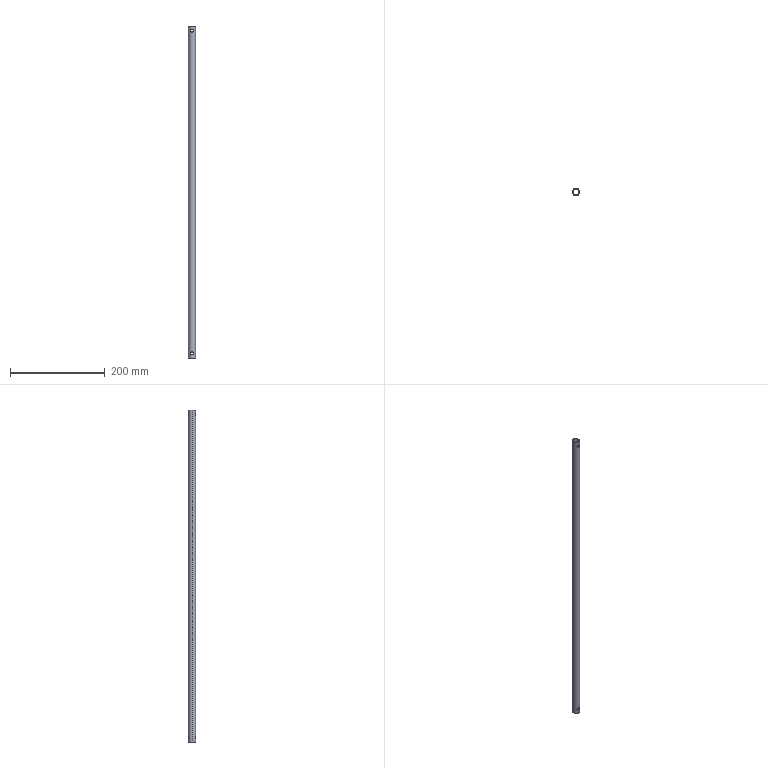Part | SolidWorks | features Extrusion 1, ICE 1 | 1 solid | 14 faces | box 15 x 15 x 700 mm | volume 44358 mm3 | cylinder 12 | plane 2 | commonest cylinder face diameters 6 x8 12 x2 15 x2
STEP:
#1=CARTESIAN_POINT('',(0.,-7.5,687.));
#2=VERTEX_POINT('',#1);
#3=CARTESIAN_POINT('',(0.,-7.5,693.));
#4=VERTEX_POINT('',#3);
#5=CARTESIAN_POINT('',(0.,-7.5,687.));
#6=CARTESIAN_POINT('',(-0.1973,-7.5,687.));
#7=CARTESIAN_POINT('',(-0.3974,-7.492,687.02));
#8=CARTESIAN_POINT('',(-0.7861,-7.461,687.098));
#9=CARTESIAN_POINT('',(-0.9739,-7.439,687.156));
#10=CARTESIAN_POINT('',(-1.337,-7.382,687.307));
#11=CARTESIAN_POINT('',(-1.511,-7.348,687.401));
#12=CARTESIAN_POINT('',(-1.834,-7.274,687.618));
#13=CARTESIAN_POINT('',(-1.985,-7.234,687.742));
#14=CARTESIAN_POINT('',(-2.261,-7.152,688.019));
#15=CARTESIAN_POINT('',(-2.384,-7.112,688.168));
#16=CARTESIAN_POINT('',(-2.6,-7.036,688.49));
#17=CARTESIAN_POINT('',(-2.694,-7.,688.665));
#18=CARTESIAN_POINT('',(-2.845,-6.94,689.027));
#19=CARTESIAN_POINT('',(-2.902,-6.916,689.214));
#20=CARTESIAN_POINT('',(-2.98,-6.883,689.601));
#21=CARTESIAN_POINT('',(-3.,-6.874,689.802));
#22=CARTESIAN_POINT('',(-3.,-6.874,690.197));
#23=CARTESIAN_POINT('',(-2.981,-6.882,690.394));
#24=CARTESIAN_POINT('',(-2.902,-6.916,690.785));
#25=CARTESIAN_POINT('',(-2.844,-6.94,690.974));
#26=CARTESIAN_POINT('',(-2.694,-7.,691.335));
#27=CARTESIAN_POINT('',(-2.6,-7.036,691.509));
#28=CARTESIAN_POINT('',(-2.383,-7.112,691.833));
#29=CARTESIAN_POINT('',(-2.26,-7.153,691.983));
#30=CARTESIAN_POINT('',(-1.985,-7.234,692.258));
#31=CARTESIAN_POINT('',(-1.833,-7.275,692.383));
#32=CARTESIAN_POINT('',(-1.51,-7.348,692.599));
#33=CARTESIAN_POINT('',(-1.339,-7.382,692.692));
#34=CARTESIAN_POINT('',(-0.9736,-7.439,692.845));
#35=CARTESIAN_POINT('',(-0.7847,-7.461,692.902));
#36=CARTESIAN_POINT('',(-0.3992,-7.492,692.98));
#37=CARTESIAN_POINT('',(-0.2004,-7.5,693.));
#38=CARTESIAN_POINT('',(0.,-7.5,693.));
#39=B_SPLINE_CURVE_WITH_KNOTS('',3,(#5,#6,#7,#8,#9,#10,#11,#12,#13,#14,#15,#16,#17,#18,#19,#20,#21,#22,#23,#24,#25,#26,#27,#28,#29,#30,#31,#32,#33,#34,#35,#36,#37,#38),.UNSPECIFIED.,.F.,.F.,(4,2,2,2,2,2,2,2,2,2,2,2,2,2,2,2,4),(0.00948,0.01007,0.01066,0.01126,0.01185,0.01244,0.01303,0.01362,0.01422,0.01481,0.0154,0.01599,0.01658,0.01718,0.01777,0.01836,0.01895),.UNSPECIFIED.);
#40=EDGE_CURVE('',#2,#4,#39,.T.);
#41=ORIENTED_EDGE('',*,*,#40,.F.);
#42=CARTESIAN_POINT('',(0.,-6.,687.));
#43=VERTEX_POINT('',#42);
#44=CARTESIAN_POINT('',(0.,-7.5,687.));
#45=DIRECTION('',(0.,1.,0.));
#46=VECTOR('',#45,1000.);
#47=LINE('',#44,#46);
#48=EDGE_CURVE('',#2,#43,#47,.T.);
#49=ORIENTED_EDGE('',*,*,#48,.T.);
#50=CARTESIAN_POINT('',(0.,-6.,693.));
#51=VERTEX_POINT('',#50);
#52=CARTESIAN_POINT('',(0.,-6.,687.));
#53=CARTESIAN_POINT('',(-0.1988,-6.,687.));
#54=CARTESIAN_POINT('',(-0.4012,-5.99,687.02));
#55=CARTESIAN_POINT('',(-0.79,-5.951,687.099));
#56=CARTESIAN_POINT('',(-0.9785,-5.923,687.157));
#57=CARTESIAN_POINT('',(-1.344,-5.851,687.311));
#58=CARTESIAN_POINT('',(-1.516,-5.808,687.404));
#59=CARTESIAN_POINT('',(-1.837,-5.714,687.62));
#60=CARTESIAN_POINT('',(-1.988,-5.663,687.745));
#61=CARTESIAN_POINT('',(-2.26,-5.56,688.018));
#62=CARTESIAN_POINT('',(-2.382,-5.508,688.166));
#63=CARTESIAN_POINT('',(-2.598,-5.409,688.488));
#64=CARTESIAN_POINT('',(-2.692,-5.363,688.662));
#65=CARTESIAN_POINT('',(-2.842,-5.285,689.02));
#66=CARTESIAN_POINT('',(-2.9,-5.253,689.207));
#67=CARTESIAN_POINT('',(-2.98,-5.208,689.599));
#68=CARTESIAN_POINT('',(-3.,-5.196,689.798));
#69=CARTESIAN_POINT('',(-3.,-5.196,690.195));
#70=CARTESIAN_POINT('',(-2.98,-5.208,690.396));
#71=CARTESIAN_POINT('',(-2.902,-5.252,690.787));
#72=CARTESIAN_POINT('',(-2.844,-5.284,690.975));
#73=CARTESIAN_POINT('',(-2.617,-5.402,691.519));
#74=CARTESIAN_POINT('',(-2.397,-5.508,691.845));
#75=CARTESIAN_POINT('',(-1.987,-5.663,692.256));
#76=CARTESIAN_POINT('',(-1.838,-5.714,692.379));
#77=CARTESIAN_POINT('',(-1.517,-5.807,692.595));
#78=CARTESIAN_POINT('',(-1.342,-5.851,692.69));
#79=CARTESIAN_POINT('',(-0.981,-5.922,692.842));
#80=CARTESIAN_POINT('',(-0.7936,-5.951,692.9));
#81=CARTESIAN_POINT('',(-0.4041,-5.99,692.979));
#82=CARTESIAN_POINT('',(-0.2015,-6.,693.));
#83=CARTESIAN_POINT('',(0.,-6.,693.));
#84=B_SPLINE_CURVE_WITH_KNOTS('',3,(#52,#53,#54,#55,#56,#57,#58,#59,#60,#61,#62,#63,#64,#65,#66,#67,#68,#69,#70,#71,#72,#73,#74,#75,#76,#77,#78,#79,#80,#81,#82,#83),.UNSPECIFIED.,.F.,.F.,(4,2,2,2,2,2,2,2,2,2,2,2,2,2,2,4),(0.009543,0.01014,0.01073,0.01133,0.01192,0.01252,0.01312,0.01371,0.01431,0.0149,0.0155,0.01669,0.01728,0.01788,0.01847,0.01907),.UNSPECIFIED.);
#85=EDGE_CURVE('',#43,#51,#84,.T.);
#86=ORIENTED_EDGE('',*,*,#85,.T.);
#87=CARTESIAN_POINT('',(0.,-7.5,693.));
#88=DIRECTION('',(0.,1.,0.));
#89=VECTOR('',#88,1000.);
#90=LINE('',#87,#89);
#91=EDGE_CURVE('',#4,#51,#90,.T.);
#92=ORIENTED_EDGE('',*,*,#91,.F.);
#93=EDGE_LOOP('',(#41,#49,#86,#92));
#94=FACE_OUTER_BOUND('',#93,.T.);
#95=CARTESIAN_POINT('',(0.,-7.5,690.));
#96=DIRECTION('',(0.,1.,0.));
#97=DIRECTION('',(0.,0.,1.));
#98=AXIS2_PLACEMENT_3D('',#95,#96,#97);
#99=CYLINDRICAL_SURFACE('',#98,3.);
#100=ADVANCED_FACE('',(#94),#99,.F.);
#101=CARTESIAN_POINT('',(0.,6.,693.));
#102=VERTEX_POINT('',#101);
#103=CARTESIAN_POINT('',(0.,6.,687.));
#104=VERTEX_POINT('',#103);
#105=CARTESIAN_POINT('',(0.,6.,693.));
#106=CARTESIAN_POINT('',(-0.2019,6.,693.));
#107=CARTESIAN_POINT('',(-0.3998,5.99,692.98));
#108=CARTESIAN_POINT('',(-0.7881,5.951,692.901));
#109=CARTESIAN_POINT('',(-0.9805,5.922,692.842));
#110=CARTESIAN_POINT('',(-1.343,5.851,692.69));
#111=CARTESIAN_POINT('',(-1.514,5.808,692.597));
#112=CARTESIAN_POINT('',(-1.838,5.714,692.379));
#113=CARTESIAN_POINT('',(-1.988,5.663,692.255));
#114=CARTESIAN_POINT('',(-2.26,5.56,691.983));
#115=CARTESIAN_POINT('',(-2.383,5.508,691.832));
#116=CARTESIAN_POINT('',(-2.6,5.409,691.51));
#117=CARTESIAN_POINT('',(-2.691,5.363,691.339));
#118=CARTESIAN_POINT('',(-2.842,5.285,690.98));
#119=CARTESIAN_POINT('',(-2.901,5.252,690.788));
#120=CARTESIAN_POINT('',(-2.98,5.208,690.399));
#121=CARTESIAN_POINT('',(-3.,5.196,690.203));
#122=CARTESIAN_POINT('',(-3.,5.196,689.803));
#123=CARTESIAN_POINT('',(-2.98,5.208,689.601));
#124=CARTESIAN_POINT('',(-2.902,5.252,689.213));
#125=CARTESIAN_POINT('',(-2.843,5.284,689.022));
#126=CARTESIAN_POINT('',(-2.691,5.363,688.659));
#127=CARTESIAN_POINT('',(-2.598,5.409,688.488));
#128=CARTESIAN_POINT('',(-2.382,5.508,688.166));
#129=CARTESIAN_POINT('',(-2.258,5.561,688.015));
#130=CARTESIAN_POINT('',(-1.985,5.664,687.743));
#131=CARTESIAN_POINT('',(-1.837,5.714,687.62));
#132=CARTESIAN_POINT('',(-1.512,5.809,687.401));
#133=CARTESIAN_POINT('',(-1.34,5.851,687.309));
#134=CARTESIAN_POINT('',(-0.9795,5.922,687.158));
#135=CARTESIAN_POINT('',(-0.789,5.951,687.099));
#136=CARTESIAN_POINT('',(-0.3968,5.99,687.02));
#137=CARTESIAN_POINT('',(-0.1992,6.,687.));
#138=CARTESIAN_POINT('',(0.,6.,687.));
#139=B_SPLINE_CURVE_WITH_KNOTS('',3,(#105,#106,#107,#108,#109,#110,#111,#112,#113,#114,#115,#116,#117,#118,#119,#120,#121,#122,#123,#124,#125,#126,#127,#128,#129,#130,#131,#132,#133,#134,#135,#136,#137,#138),.UNSPECIFIED.,.F.,.F.,(4,2,2,2,2,2,2,2,2,2,2,2,2,2,2,2,4),(0.,0.0005964,0.001193,0.001789,0.002386,0.002982,0.003579,0.004175,0.004771,0.005368,0.005964,0.006561,0.007157,0.007754,0.00835,0.008947,0.009543),.UNSPECIFIED.);
#140=EDGE_CURVE('',#102,#104,#139,.T.);
#141=ORIENTED_EDGE('',*,*,#140,.T.);
#142=CARTESIAN_POINT('',(0.,7.5,687.));
#143=VERTEX_POINT('',#142);
#144=CARTESIAN_POINT('',(0.,-7.5,687.));
#145=DIRECTION('',(0.,1.,0.));
#146=VECTOR('',#145,1000.);
#147=LINE('',#144,#146);
#148=EDGE_CURVE('',#104,#143,#147,.T.);
#149=ORIENTED_EDGE('',*,*,#148,.T.);
#150=CARTESIAN_POINT('',(0.,7.5,693.));
#151=VERTEX_POINT('',#150);
#152=CARTESIAN_POINT('',(0.,7.5,693.));
#153=CARTESIAN_POINT('',(-0.2005,7.5,693.));
#154=CARTESIAN_POINT('',(-0.3972,7.492,692.98));
#155=CARTESIAN_POINT('',(-0.7836,7.461,692.903));
#156=CARTESIAN_POINT('',(-0.9753,7.439,692.844));
#157=CARTESIAN_POINT('',(-1.338,7.382,692.692));
#158=CARTESIAN_POINT('',(-1.509,7.348,692.6));
#159=CARTESIAN_POINT('',(-1.834,7.274,692.382));
#160=CARTESIAN_POINT('',(-1.986,7.234,692.257));
#161=CARTESIAN_POINT('',(-2.396,7.113,691.846));
#162=CARTESIAN_POINT('',(-2.618,7.03,691.515));
#163=CARTESIAN_POINT('',(-2.844,6.94,690.975));
#164=CARTESIAN_POINT('',(-2.902,6.916,690.784));
#165=CARTESIAN_POINT('',(-2.98,6.883,690.396));
#166=CARTESIAN_POINT('',(-3.,6.874,690.2));
#167=CARTESIAN_POINT('',(-3.,6.874,689.804));
#168=CARTESIAN_POINT('',(-2.98,6.883,689.603));
#169=CARTESIAN_POINT('',(-2.902,6.916,689.216));
#170=CARTESIAN_POINT('',(-2.845,6.94,689.028));
#171=CARTESIAN_POINT('',(-2.692,7.001,688.662));
#172=CARTESIAN_POINT('',(-2.6,7.036,688.491));
#173=CARTESIAN_POINT('',(-2.383,7.112,688.168));
#174=CARTESIAN_POINT('',(-2.258,7.153,688.015));
#175=CARTESIAN_POINT('',(-1.983,7.234,687.741));
#176=CARTESIAN_POINT('',(-1.834,7.274,687.618));
#177=CARTESIAN_POINT('',(-1.51,7.348,687.4));
#178=CARTESIAN_POINT('',(-1.335,7.383,687.306));
#179=CARTESIAN_POINT('',(-0.974,7.439,687.156));
#180=CARTESIAN_POINT('',(-0.7864,7.461,687.098));
#181=CARTESIAN_POINT('',(-0.3955,7.492,687.02));
#182=CARTESIAN_POINT('',(-0.1975,7.5,687.));
#183=CARTESIAN_POINT('',(0.,7.5,687.));
#184=B_SPLINE_CURVE_WITH_KNOTS('',3,(#152,#153,#154,#155,#156,#157,#158,#159,#160,#161,#162,#163,#164,#165,#166,#167,#168,#169,#170,#171,#172,#173,#174,#175,#176,#177,#178,#179,#180,#181,#182,#183),.UNSPECIFIED.,.F.,.F.,(4,2,2,2,2,2,2,2,2,2,2,2,2,2,2,4),(0.,0.0005925,0.001185,0.001777,0.00237,0.003555,0.004147,0.00474,0.005332,0.005925,0.006517,0.00711,0.007702,0.008295,0.008887,0.00948),.UNSPECIFIED.);
#185=EDGE_CURVE('',#151,#143,#184,.T.);
#186=ORIENTED_EDGE('',*,*,#185,.F.);
#187=CARTESIAN_POINT('',(0.,-7.5,693.));
#188=DIRECTION('',(0.,1.,0.));
#189=VECTOR('',#188,1000.);
#190=LINE('',#187,#189);
#191=EDGE_CURVE('',#102,#151,#190,.T.);
#192=ORIENTED_EDGE('',*,*,#191,.F.);
#193=EDGE_LOOP('',(#141,#149,#186,#192));
#194=FACE_OUTER_BOUND('',#193,.T.);
#195=CARTESIAN_POINT('',(0.,-7.5,690.));
#196=DIRECTION('',(0.,1.,0.));
#197=DIRECTION('',(0.,0.,1.));
#198=AXIS2_PLACEMENT_3D('',#195,#196,#197);
#199=CYLINDRICAL_SURFACE('',#198,3.);
#200=ADVANCED_FACE('',(#194),#199,.F.);
#201=CARTESIAN_POINT('',(0.,-7.5,7.));
#202=VERTEX_POINT('',#201);
#203=CARTESIAN_POINT('',(0.,-7.5,13.));
#204=VERTEX_POINT('',#203);
#205=CARTESIAN_POINT('',(0.,-7.5,7.));
#206=CARTESIAN_POINT('',(-0.1973,-7.5,7.));
#207=CARTESIAN_POINT('',(-0.3974,-7.492,7.02));
#208=CARTESIAN_POINT('',(-0.7861,-7.461,7.098));
#209=CARTESIAN_POINT('',(-0.9739,-7.439,7.156));
#210=CARTESIAN_POINT('',(-1.337,-7.382,7.307));
#211=CARTESIAN_POINT('',(-1.511,-7.348,7.401));
#212=CARTESIAN_POINT('',(-1.834,-7.274,7.618));
#213=CARTESIAN_POINT('',(-1.985,-7.234,7.742));
#214=CARTESIAN_POINT('',(-2.261,-7.152,8.019));
#215=CARTESIAN_POINT('',(-2.384,-7.112,8.168));
#216=CARTESIAN_POINT('',(-2.6,-7.036,8.49));
#217=CARTESIAN_POINT('',(-2.694,-7.,8.665));
#218=CARTESIAN_POINT('',(-2.845,-6.94,9.027));
#219=CARTESIAN_POINT('',(-2.902,-6.916,9.214));
#220=CARTESIAN_POINT('',(-2.98,-6.883,9.601));
#221=CARTESIAN_POINT('',(-3.,-6.874,9.802));
#222=CARTESIAN_POINT('',(-3.,-6.874,10.197));
#223=CARTESIAN_POINT('',(-2.981,-6.882,10.394));
#224=CARTESIAN_POINT('',(-2.902,-6.916,10.785));
#225=CARTESIAN_POINT('',(-2.844,-6.94,10.974));
#226=CARTESIAN_POINT('',(-2.694,-7.,11.335));
#227=CARTESIAN_POINT('',(-2.6,-7.036,11.509));
#228=CARTESIAN_POINT('',(-2.383,-7.112,11.833));
#229=CARTESIAN_POINT('',(-2.26,-7.153,11.983));
#230=CARTESIAN_POINT('',(-1.985,-7.234,12.258));
#231=CARTESIAN_POINT('',(-1.833,-7.275,12.383));
#232=CARTESIAN_POINT('',(-1.51,-7.348,12.599));
#233=CARTESIAN_POINT('',(-1.339,-7.382,12.692));
#234=CARTESIAN_POINT('',(-0.9736,-7.439,12.845));
#235=CARTESIAN_POINT('',(-0.7847,-7.461,12.902));
#236=CARTESIAN_POINT('',(-0.3992,-7.492,12.98));
#237=CARTESIAN_POINT('',(-0.2004,-7.5,13.));
#238=CARTESIAN_POINT('',(0.,-7.5,13.));
#239=B_SPLINE_CURVE_WITH_KNOTS('',3,(#205,#206,#207,#208,#209,#210,#211,#212,#213,#214,#215,#216,#217,#218,#219,#220,#221,#222,#223,#224,#225,#226,#227,#228,#229,#230,#231,#232,#233,#234,#235,#236,#237,#238),.UNSPECIFIED.,.F.,.F.,(4,2,2,2,2,2,2,2,2,2,2,2,2,2,2,2,4),(0.00948,0.01007,0.01066,0.01126,0.01185,0.01244,0.01303,0.01362,0.01422,0.01481,0.0154,0.01599,0.01658,0.01718,0.01777,0.01836,0.01895),.UNSPECIFIED.);
#240=EDGE_CURVE('',#202,#204,#239,.T.);
#241=ORIENTED_EDGE('',*,*,#240,.F.);
#242=CARTESIAN_POINT('',(0.,-6.,7.));
#243=VERTEX_POINT('',#242);
#244=CARTESIAN_POINT('',(0.,-7.5,7.));
#245=DIRECTION('',(0.,1.,0.));
#246=VECTOR('',#245,1000.);
#247=LINE('',#244,#246);
#248=EDGE_CURVE('',#202,#243,#247,.T.);
#249=ORIENTED_EDGE('',*,*,#248,.T.);
#250=CARTESIAN_POINT('',(0.,-6.,13.));
#251=VERTEX_POINT('',#250);
#252=CARTESIAN_POINT('',(0.,-6.,7.));
#253=CARTESIAN_POINT('',(-0.1988,-6.,7.));
#254=CARTESIAN_POINT('',(-0.4012,-5.99,7.02));
#255=CARTESIAN_POINT('',(-0.79,-5.951,7.099));
#256=CARTESIAN_POINT('',(-0.9785,-5.923,7.157));
#257=CARTESIAN_POINT('',(-1.344,-5.851,7.311));
#258=CARTESIAN_POINT('',(-1.516,-5.808,7.404));
#259=CARTESIAN_POINT('',(-1.837,-5.714,7.62));
#260=CARTESIAN_POINT('',(-1.988,-5.663,7.745));
#261=CARTESIAN_POINT('',(-2.26,-5.56,8.018));
#262=CARTESIAN_POINT('',(-2.382,-5.508,8.166));
#263=CARTESIAN_POINT('',(-2.598,-5.409,8.488));
#264=CARTESIAN_POINT('',(-2.692,-5.363,8.662));
#265=CARTESIAN_POINT('',(-2.842,-5.285,9.02));
#266=CARTESIAN_POINT('',(-2.9,-5.253,9.207));
#267=CARTESIAN_POINT('',(-2.98,-5.208,9.599));
#268=CARTESIAN_POINT('',(-3.,-5.196,9.798));
#269=CARTESIAN_POINT('',(-3.,-5.196,10.195));
#270=CARTESIAN_POINT('',(-2.98,-5.208,10.396));
#271=CARTESIAN_POINT('',(-2.902,-5.252,10.787));
#272=CARTESIAN_POINT('',(-2.844,-5.284,10.975));
#273=CARTESIAN_POINT('',(-2.617,-5.402,11.519));
#274=CARTESIAN_POINT('',(-2.397,-5.508,11.845));
#275=CARTESIAN_POINT('',(-1.987,-5.663,12.256));
#276=CARTESIAN_POINT('',(-1.838,-5.714,12.379));
#277=CARTESIAN_POINT('',(-1.517,-5.807,12.595));
#278=CARTESIAN_POINT('',(-1.342,-5.851,12.69));
#279=CARTESIAN_POINT('',(-0.981,-5.922,12.842));
#280=CARTESIAN_POINT('',(-0.7936,-5.951,12.9));
#281=CARTESIAN_POINT('',(-0.4041,-5.99,12.979));
#282=CARTESIAN_POINT('',(-0.2015,-6.,13.));
#283=CARTESIAN_POINT('',(0.,-6.,13.));
#284=B_SPLINE_CURVE_WITH_KNOTS('',3,(#252,#253,#254,#255,#256,#257,#258,#259,#260,#261,#262,#263,#264,#265,#266,#267,#268,#269,#270,#271,#272,#273,#274,#275,#276,#277,#278,#279,#280,#281,#282,#283),.UNSPECIFIED.,.F.,.F.,(4,2,2,2,2,2,2,2,2,2,2,2,2,2,2,4),(0.009543,0.01014,0.01073,0.01133,0.01192,0.01252,0.01312,0.01371,0.01431,0.0149,0.0155,0.01669,0.01728,0.01788,0.01847,0.01907),.UNSPECIFIED.);
#285=EDGE_CURVE('',#243,#251,#284,.T.);
#286=ORIENTED_EDGE('',*,*,#285,.T.);
#287=CARTESIAN_POINT('',(0.,-7.5,13.));
#288=DIRECTION('',(0.,1.,0.));
#289=VECTOR('',#288,1000.);
#290=LINE('',#287,#289);
#291=EDGE_CURVE('',#204,#251,#290,.T.);
#292=ORIENTED_EDGE('',*,*,#291,.F.);
#293=EDGE_LOOP('',(#241,#249,#286,#292));
#294=FACE_OUTER_BOUND('',#293,.T.);
#295=CARTESIAN_POINT('',(0.,-7.5,10.));
#296=DIRECTION('',(0.,1.,0.));
#297=DIRECTION('',(0.,0.,1.));
#298=AXIS2_PLACEMENT_3D('',#295,#296,#297);
#299=CYLINDRICAL_SURFACE('',#298,3.);
#300=ADVANCED_FACE('',(#294),#299,.F.);
#301=CARTESIAN_POINT('',(0.,6.,13.));
#302=VERTEX_POINT('',#301);
#303=CARTESIAN_POINT('',(0.,6.,7.));
#304=VERTEX_POINT('',#303);
#305=CARTESIAN_POINT('',(0.,6.,13.));
#306=CARTESIAN_POINT('',(-0.2019,6.,13.));
#307=CARTESIAN_POINT('',(-0.3998,5.99,12.98));
#308=CARTESIAN_POINT('',(-0.7881,5.951,12.901));
#309=CARTESIAN_POINT('',(-0.9805,5.922,12.842));
#310=CARTESIAN_POINT('',(-1.343,5.851,12.69));
#311=CARTESIAN_POINT('',(-1.514,5.808,12.597));
#312=CARTESIAN_POINT('',(-1.838,5.714,12.379));
#313=CARTESIAN_POINT('',(-1.988,5.663,12.255));
#314=CARTESIAN_POINT('',(-2.26,5.56,11.983));
#315=CARTESIAN_POINT('',(-2.383,5.508,11.832));
#316=CARTESIAN_POINT('',(-2.6,5.409,11.51));
#317=CARTESIAN_POINT('',(-2.691,5.363,11.339));
#318=CARTESIAN_POINT('',(-2.842,5.285,10.98));
#319=CARTESIAN_POINT('',(-2.901,5.252,10.788));
#320=CARTESIAN_POINT('',(-2.98,5.208,10.399));
#321=CARTESIAN_POINT('',(-3.,5.196,10.203));
#322=CARTESIAN_POINT('',(-3.,5.196,9.803));
#323=CARTESIAN_POINT('',(-2.98,5.208,9.601));
#324=CARTESIAN_POINT('',(-2.902,5.252,9.213));
#325=CARTESIAN_POINT('',(-2.843,5.284,9.022));
#326=CARTESIAN_POINT('',(-2.691,5.363,8.659));
#327=CARTESIAN_POINT('',(-2.598,5.409,8.488));
#328=CARTESIAN_POINT('',(-2.382,5.508,8.166));
#329=CARTESIAN_POINT('',(-2.258,5.561,8.015));
#330=CARTESIAN_POINT('',(-1.985,5.664,7.743));
#331=CARTESIAN_POINT('',(-1.837,5.714,7.62));
#332=CARTESIAN_POINT('',(-1.512,5.809,7.401));
#333=CARTESIAN_POINT('',(-1.34,5.851,7.309));
#334=CARTESIAN_POINT('',(-0.9795,5.922,7.158));
#335=CARTESIAN_POINT('',(-0.789,5.951,7.099));
#336=CARTESIAN_POINT('',(-0.3968,5.99,7.02));
#337=CARTESIAN_POINT('',(-0.1992,6.,7.));
#338=CARTESIAN_POINT('',(0.,6.,7.));
#339=B_SPLINE_CURVE_WITH_KNOTS('',3,(#305,#306,#307,#308,#309,#310,#311,#312,#313,#314,#315,#316,#317,#318,#319,#320,#321,#322,#323,#324,#325,#326,#327,#328,#329,#330,#331,#332,#333,#334,#335,#336,#337,#338),.UNSPECIFIED.,.F.,.F.,(4,2,2,2,2,2,2,2,2,2,2,2,2,2,2,2,4),(0.,0.0005964,0.001193,0.001789,0.002386,0.002982,0.003579,0.004175,0.004771,0.005368,0.005964,0.006561,0.007157,0.007754,0.00835,0.008947,0.009543),.UNSPECIFIED.);
#340=EDGE_CURVE('',#302,#304,#339,.T.);
#341=ORIENTED_EDGE('',*,*,#340,.T.);
#342=CARTESIAN_POINT('',(0.,7.5,7.));
#343=VERTEX_POINT('',#342);
#344=CARTESIAN_POINT('',(0.,-7.5,7.));
#345=DIRECTION('',(0.,1.,0.));
#346=VECTOR('',#345,1000.);
#347=LINE('',#344,#346);
#348=EDGE_CURVE('',#304,#343,#347,.T.);
#349=ORIENTED_EDGE('',*,*,#348,.T.);
#350=CARTESIAN_POINT('',(0.,7.5,13.));
#351=VERTEX_POINT('',#350);
#352=CARTESIAN_POINT('',(0.,7.5,13.));
#353=CARTESIAN_POINT('',(-0.2005,7.5,13.));
#354=CARTESIAN_POINT('',(-0.3972,7.492,12.98));
#355=CARTESIAN_POINT('',(-0.7836,7.461,12.903));
#356=CARTESIAN_POINT('',(-0.9753,7.439,12.844));
#357=CARTESIAN_POINT('',(-1.338,7.382,12.692));
#358=CARTESIAN_POINT('',(-1.509,7.348,12.6));
#359=CARTESIAN_POINT('',(-1.834,7.274,12.382));
#360=CARTESIAN_POINT('',(-1.986,7.234,12.257));
#361=CARTESIAN_POINT('',(-2.396,7.113,11.846));
#362=CARTESIAN_POINT('',(-2.618,7.03,11.515));
#363=CARTESIAN_POINT('',(-2.844,6.94,10.975));
#364=CARTESIAN_POINT('',(-2.902,6.916,10.784));
#365=CARTESIAN_POINT('',(-2.98,6.883,10.396));
#366=CARTESIAN_POINT('',(-3.,6.874,10.2));
#367=CARTESIAN_POINT('',(-3.,6.874,9.804));
#368=CARTESIAN_POINT('',(-2.98,6.883,9.603));
#369=CARTESIAN_POINT('',(-2.902,6.916,9.216));
#370=CARTESIAN_POINT('',(-2.845,6.94,9.028));
#371=CARTESIAN_POINT('',(-2.692,7.001,8.662));
#372=CARTESIAN_POINT('',(-2.6,7.036,8.491));
#373=CARTESIAN_POINT('',(-2.383,7.112,8.168));
#374=CARTESIAN_POINT('',(-2.258,7.153,8.015));
#375=CARTESIAN_POINT('',(-1.983,7.234,7.741));
#376=CARTESIAN_POINT('',(-1.834,7.274,7.618));
#377=CARTESIAN_POINT('',(-1.51,7.348,7.4));
#378=CARTESIAN_POINT('',(-1.335,7.383,7.306));
#379=CARTESIAN_POINT('',(-0.974,7.439,7.156));
#380=CARTESIAN_POINT('',(-0.7864,7.461,7.098));
#381=CARTESIAN_POINT('',(-0.3955,7.492,7.02));
#382=CARTESIAN_POINT('',(-0.1975,7.5,7.));
#383=CARTESIAN_POINT('',(0.,7.5,7.));
#384=B_SPLINE_CURVE_WITH_KNOTS('',3,(#352,#353,#354,#355,#356,#357,#358,#359,#360,#361,#362,#363,#364,#365,#366,#367,#368,#369,#370,#371,#372,#373,#374,#375,#376,#377,#378,#379,#380,#381,#382,#383),.UNSPECIFIED.,.F.,.F.,(4,2,2,2,2,2,2,2,2,2,2,2,2,2,2,4),(0.,0.0005925,0.001185,0.001777,0.00237,0.003555,0.004147,0.00474,0.005332,0.005925,0.006517,0.00711,0.007702,0.008295,0.008887,0.00948),.UNSPECIFIED.);
#385=EDGE_CURVE('',#351,#343,#384,.T.);
#386=ORIENTED_EDGE('',*,*,#385,.F.);
#387=CARTESIAN_POINT('',(0.,-7.5,13.));
#388=DIRECTION('',(0.,1.,0.));
#389=VECTOR('',#388,1000.);
#390=LINE('',#387,#389);
#391=EDGE_CURVE('',#302,#351,#390,.T.);
#392=ORIENTED_EDGE('',*,*,#391,.F.);
#393=EDGE_LOOP('',(#341,#349,#386,#392));
#394=FACE_OUTER_BOUND('',#393,.T.);
#395=CARTESIAN_POINT('',(0.,-7.5,10.));
#396=DIRECTION('',(0.,1.,0.));
#397=DIRECTION('',(0.,0.,1.));
#398=AXIS2_PLACEMENT_3D('',#395,#396,#397);
#399=CYLINDRICAL_SURFACE('',#398,3.);
#400=ADVANCED_FACE('',(#394),#399,.F.);
#401=CARTESIAN_POINT('',(0.,-6.,13.));
#402=CARTESIAN_POINT('',(0.2019,-6.,13.));
#403=CARTESIAN_POINT('',(0.3998,-5.99,12.98));
#404=CARTESIAN_POINT('',(0.7881,-5.951,12.901));
#405=CARTESIAN_POINT('',(0.9805,-5.922,12.842));
#406=CARTESIAN_POINT('',(1.343,-5.851,12.69));
#407=CARTESIAN_POINT('',(1.514,-5.808,12.597));
#408=CARTESIAN_POINT('',(1.838,-5.714,12.379));
#409=CARTESIAN_POINT('',(1.988,-5.663,12.255));
#410=CARTESIAN_POINT('',(2.26,-5.56,11.983));
#411=CARTESIAN_POINT('',(2.383,-5.508,11.832));
#412=CARTESIAN_POINT('',(2.6,-5.409,11.51));
#413=CARTESIAN_POINT('',(2.691,-5.363,11.339));
#414=CARTESIAN_POINT('',(2.842,-5.285,10.98));
#415=CARTESIAN_POINT('',(2.901,-5.252,10.788));
#416=CARTESIAN_POINT('',(2.98,-5.208,10.399));
#417=CARTESIAN_POINT('',(3.,-5.196,10.203));
#418=CARTESIAN_POINT('',(3.,-5.196,9.803));
#419=CARTESIAN_POINT('',(2.98,-5.208,9.601));
#420=CARTESIAN_POINT('',(2.902,-5.252,9.213));
#421=CARTESIAN_POINT('',(2.843,-5.284,9.022));
#422=CARTESIAN_POINT('',(2.691,-5.363,8.659));
#423=CARTESIAN_POINT('',(2.598,-5.409,8.488));
#424=CARTESIAN_POINT('',(2.382,-5.508,8.166));
#425=CARTESIAN_POINT('',(2.258,-5.561,8.015));
#426=CARTESIAN_POINT('',(1.985,-5.664,7.743));
#427=CARTESIAN_POINT('',(1.837,-5.714,7.62));
#428=CARTESIAN_POINT('',(1.512,-5.809,7.401));
#429=CARTESIAN_POINT('',(1.34,-5.851,7.309));
#430=CARTESIAN_POINT('',(0.9795,-5.922,7.158));
#431=CARTESIAN_POINT('',(0.789,-5.951,7.099));
#432=CARTESIAN_POINT('',(0.3968,-5.99,7.02));
#433=CARTESIAN_POINT('',(0.1992,-6.,7.));
#434=CARTESIAN_POINT('',(0.,-6.,7.));
#435=B_SPLINE_CURVE_WITH_KNOTS('',3,(#401,#402,#403,#404,#405,#406,#407,#408,#409,#410,#411,#412,#413,#414,#415,#416,#417,#418,#419,#420,#421,#422,#423,#424,#425,#426,#427,#428,#429,#430,#431,#432,#433,#434),.UNSPECIFIED.,.F.,.F.,(4,2,2,2,2,2,2,2,2,2,2,2,2,2,2,2,4),(0.,0.0005964,0.001193,0.001789,0.002386,0.002982,0.003579,0.004175,0.004771,0.005368,0.005964,0.006561,0.007157,0.007754,0.00835,0.008947,0.009543),.UNSPECIFIED.);
#436=EDGE_CURVE('',#251,#243,#435,.T.);
#437=ORIENTED_EDGE('',*,*,#436,.F.);
#438=ORIENTED_EDGE('',*,*,#285,.F.);
#439=EDGE_LOOP('',(#437,#438));
#440=FACE_BOUND('',#439,.T.);
#441=CARTESIAN_POINT('',(0.,-6.,693.));
#442=CARTESIAN_POINT('',(0.2019,-6.,693.));
#443=CARTESIAN_POINT('',(0.3998,-5.99,692.98));
#444=CARTESIAN_POINT('',(0.7881,-5.951,692.901));
#445=CARTESIAN_POINT('',(0.9805,-5.922,692.842));
#446=CARTESIAN_POINT('',(1.343,-5.851,692.69));
#447=CARTESIAN_POINT('',(1.514,-5.808,692.597));
#448=CARTESIAN_POINT('',(1.838,-5.714,692.379));
#449=CARTESIAN_POINT('',(1.988,-5.663,692.255));
#450=CARTESIAN_POINT('',(2.26,-5.56,691.983));
#451=CARTESIAN_POINT('',(2.383,-5.508,691.832));
#452=CARTESIAN_POINT('',(2.6,-5.409,691.51));
#453=CARTESIAN_POINT('',(2.691,-5.363,691.339));
#454=CARTESIAN_POINT('',(2.842,-5.285,690.98));
#455=CARTESIAN_POINT('',(2.901,-5.252,690.788));
#456=CARTESIAN_POINT('',(2.98,-5.208,690.399));
#457=CARTESIAN_POINT('',(3.,-5.196,690.203));
#458=CARTESIAN_POINT('',(3.,-5.196,689.803));
#459=CARTESIAN_POINT('',(2.98,-5.208,689.601));
#460=CARTESIAN_POINT('',(2.902,-5.252,689.213));
#461=CARTESIAN_POINT('',(2.843,-5.284,689.022));
#462=CARTESIAN_POINT('',(2.691,-5.363,688.659));
#463=CARTESIAN_POINT('',(2.598,-5.409,688.488));
#464=CARTESIAN_POINT('',(2.382,-5.508,688.166));
#465=CARTESIAN_POINT('',(2.258,-5.561,688.015));
#466=CARTESIAN_POINT('',(1.985,-5.664,687.743));
#467=CARTESIAN_POINT('',(1.837,-5.714,687.62));
#468=CARTESIAN_POINT('',(1.512,-5.809,687.401));
#469=CARTESIAN_POINT('',(1.34,-5.851,687.309));
#470=CARTESIAN_POINT('',(0.9795,-5.922,687.158));
#471=CARTESIAN_POINT('',(0.789,-5.951,687.099));
#472=CARTESIAN_POINT('',(0.3968,-5.99,687.02));
#473=CARTESIAN_POINT('',(0.1992,-6.,687.));
#474=CARTESIAN_POINT('',(0.,-6.,687.));
#475=B_SPLINE_CURVE_WITH_KNOTS('',3,(#441,#442,#443,#444,#445,#446,#447,#448,#449,#450,#451,#452,#453,#454,#455,#456,#457,#458,#459,#460,#461,#462,#463,#464,#465,#466,#467,#468,#469,#470,#471,#472,#473,#474),.UNSPECIFIED.,.F.,.F.,(4,2,2,2,2,2,2,2,2,2,2,2,2,2,2,2,4),(0.,0.0005964,0.001193,0.001789,0.002386,0.002982,0.003579,0.004175,0.004771,0.005368,0.005964,0.006561,0.007157,0.007754,0.00835,0.008947,0.009543),.UNSPECIFIED.);
#476=EDGE_CURVE('',#51,#43,#475,.T.);
#477=ORIENTED_EDGE('',*,*,#476,.F.);
#478=ORIENTED_EDGE('',*,*,#85,.F.);
#479=EDGE_LOOP('',(#477,#478));
#480=FACE_BOUND('',#479,.T.);
#481=CARTESIAN_POINT('',(-6.,0.,700.));
#482=VERTEX_POINT('',#481);
#483=CARTESIAN_POINT('',(6.,0.,700.));
#484=VERTEX_POINT('',#483);
#485=CARTESIAN_POINT('',(0.,0.,700.));
#486=DIRECTION('',(0.,0.,1.));
#487=DIRECTION('',(1.,0.,0.));
#488=AXIS2_PLACEMENT_3D('',#485,#486,#487);
#489=CIRCLE('',#488,6.);
#490=EDGE_CURVE('',#482,#484,#489,.T.);
#491=ORIENTED_EDGE('',*,*,#490,.T.);
#492=CARTESIAN_POINT('',(6.,0.,0.));
#493=VERTEX_POINT('',#492);
#494=CARTESIAN_POINT('',(6.,0.,700.));
#495=DIRECTION('',(0.,0.,-1.));
#496=VECTOR('',#495,1000.);
#497=LINE('',#494,#496);
#498=EDGE_CURVE('',#484,#493,#497,.T.);
#499=ORIENTED_EDGE('',*,*,#498,.T.);
#500=CARTESIAN_POINT('',(-6.,0.,0.));
#501=VERTEX_POINT('',#500);
#502=CARTESIAN_POINT('',(0.,0.,0.));
#503=DIRECTION('',(0.,0.,1.));
#504=DIRECTION('',(1.,0.,0.));
#505=AXIS2_PLACEMENT_3D('',#502,#503,#504);
#506=CIRCLE('',#505,6.);
#507=EDGE_CURVE('',#501,#493,#506,.T.);
#508=ORIENTED_EDGE('',*,*,#507,.F.);
#509=CARTESIAN_POINT('',(-6.,0.,700.));
#510=DIRECTION('',(0.,0.,-1.));
#511=VECTOR('',#510,1000.);
#512=LINE('',#509,#511);
#513=EDGE_CURVE('',#482,#501,#512,.T.);
#514=ORIENTED_EDGE('',*,*,#513,.F.);
#515=EDGE_LOOP('',(#491,#499,#508,#514));
#516=FACE_OUTER_BOUND('',#515,.T.);
#517=CARTESIAN_POINT('',(0.,0.,700.));
#518=DIRECTION('',(0.,0.,-1.));
#519=DIRECTION('',(-1.,0.,0.));
#520=AXIS2_PLACEMENT_3D('',#517,#518,#519);
#521=CYLINDRICAL_SURFACE('',#520,6.);
#522=ADVANCED_FACE('',(#440,#480,#516),#521,.F.);
#523=ORIENTED_EDGE('',*,*,#385,.T.);
#524=CARTESIAN_POINT('',(0.,7.5,7.));
#525=CARTESIAN_POINT('',(0.1973,7.5,7.));
#526=CARTESIAN_POINT('',(0.3974,7.492,7.02));
#527=CARTESIAN_POINT('',(0.7861,7.461,7.098));
#528=CARTESIAN_POINT('',(0.9739,7.439,7.156));
#529=CARTESIAN_POINT('',(1.337,7.382,7.307));
#530=CARTESIAN_POINT('',(1.511,7.348,7.401));
#531=CARTESIAN_POINT('',(1.834,7.274,7.618));
#532=CARTESIAN_POINT('',(1.985,7.234,7.742));
#533=CARTESIAN_POINT('',(2.261,7.152,8.019));
#534=CARTESIAN_POINT('',(2.384,7.112,8.168));
#535=CARTESIAN_POINT('',(2.6,7.036,8.49));
#536=CARTESIAN_POINT('',(2.694,7.,8.665));
#537=CARTESIAN_POINT('',(2.845,6.94,9.027));
#538=CARTESIAN_POINT('',(2.902,6.916,9.214));
#539=CARTESIAN_POINT('',(2.98,6.883,9.601));
#540=CARTESIAN_POINT('',(3.,6.874,9.802));
#541=CARTESIAN_POINT('',(3.,6.874,10.197));
#542=CARTESIAN_POINT('',(2.981,6.882,10.394));
#543=CARTESIAN_POINT('',(2.902,6.916,10.785));
#544=CARTESIAN_POINT('',(2.844,6.94,10.974));
#545=CARTESIAN_POINT('',(2.694,7.,11.335));
#546=CARTESIAN_POINT('',(2.6,7.036,11.509));
#547=CARTESIAN_POINT('',(2.383,7.112,11.833));
#548=CARTESIAN_POINT('',(2.26,7.153,11.983));
#549=CARTESIAN_POINT('',(1.985,7.234,12.258));
#550=CARTESIAN_POINT('',(1.833,7.275,12.383));
#551=CARTESIAN_POINT('',(1.51,7.348,12.599));
#552=CARTESIAN_POINT('',(1.339,7.382,12.692));
#553=CARTESIAN_POINT('',(0.9736,7.439,12.845));
#554=CARTESIAN_POINT('',(0.7847,7.461,12.902));
#555=CARTESIAN_POINT('',(0.3992,7.492,12.98));
#556=CARTESIAN_POINT('',(0.2004,7.5,13.));
#557=CARTESIAN_POINT('',(0.,7.5,13.));
#558=B_SPLINE_CURVE_WITH_KNOTS('',3,(#524,#525,#526,#527,#528,#529,#530,#531,#532,#533,#534,#535,#536,#537,#538,#539,#540,#541,#542,#543,#544,#545,#546,#547,#548,#549,#550,#551,#552,#553,#554,#555,#556,#557),.UNSPECIFIED.,.F.,.F.,(4,2,2,2,2,2,2,2,2,2,2,2,2,2,2,2,4),(0.00948,0.01007,0.01066,0.01126,0.01185,0.01244,0.01303,0.01362,0.01422,0.01481,0.0154,0.01599,0.01658,0.01718,0.01777,0.01836,0.01895),.UNSPECIFIED.);
#559=EDGE_CURVE('',#343,#351,#558,.T.);
#560=ORIENTED_EDGE('',*,*,#559,.T.);
#561=EDGE_LOOP('',(#523,#560));
#562=FACE_BOUND('',#561,.T.);
#563=ORIENTED_EDGE('',*,*,#185,.T.);
#564=CARTESIAN_POINT('',(0.,7.5,687.));
#565=CARTESIAN_POINT('',(0.1973,7.5,687.));
#566=CARTESIAN_POINT('',(0.3974,7.492,687.02));
#567=CARTESIAN_POINT('',(0.7861,7.461,687.098));
#568=CARTESIAN_POINT('',(0.9739,7.439,687.156));
#569=CARTESIAN_POINT('',(1.337,7.382,687.307));
#570=CARTESIAN_POINT('',(1.511,7.348,687.401));
#571=CARTESIAN_POINT('',(1.834,7.274,687.618));
#572=CARTESIAN_POINT('',(1.985,7.234,687.742));
#573=CARTESIAN_POINT('',(2.261,7.152,688.019));
#574=CARTESIAN_POINT('',(2.384,7.112,688.168));
#575=CARTESIAN_POINT('',(2.6,7.036,688.49));
#576=CARTESIAN_POINT('',(2.694,7.,688.665));
#577=CARTESIAN_POINT('',(2.845,6.94,689.027));
#578=CARTESIAN_POINT('',(2.902,6.916,689.214));
#579=CARTESIAN_POINT('',(2.98,6.883,689.601));
#580=CARTESIAN_POINT('',(3.,6.874,689.802));
#581=CARTESIAN_POINT('',(3.,6.874,690.197));
#582=CARTESIAN_POINT('',(2.981,6.882,690.394));
#583=CARTESIAN_POINT('',(2.902,6.916,690.785));
#584=CARTESIAN_POINT('',(2.844,6.94,690.974));
#585=CARTESIAN_POINT('',(2.694,7.,691.335));
#586=CARTESIAN_POINT('',(2.6,7.036,691.509));
#587=CARTESIAN_POINT('',(2.383,7.112,691.833));
#588=CARTESIAN_POINT('',(2.26,7.153,691.983));
#589=CARTESIAN_POINT('',(1.985,7.234,692.258));
#590=CARTESIAN_POINT('',(1.833,7.275,692.383));
#591=CARTESIAN_POINT('',(1.51,7.348,692.599));
#592=CARTESIAN_POINT('',(1.339,7.382,692.692));
#593=CARTESIAN_POINT('',(0.9736,7.439,692.845));
#594=CARTESIAN_POINT('',(0.7847,7.461,692.902));
#595=CARTESIAN_POINT('',(0.3992,7.492,692.98));
#596=CARTESIAN_POINT('',(0.2004,7.5,693.));
#597=CARTESIAN_POINT('',(0.,7.5,693.));
#598=B_SPLINE_CURVE_WITH_KNOTS('',3,(#564,#565,#566,#567,#568,#569,#570,#571,#572,#573,#574,#575,#576,#577,#578,#579,#580,#581,#582,#583,#584,#585,#586,#587,#588,#589,#590,#591,#592,#593,#594,#595,#596,#597),.UNSPECIFIED.,.F.,.F.,(4,2,2,2,2,2,2,2,2,2,2,2,2,2,2,2,4),(0.00948,0.01007,0.01066,0.01126,0.01185,0.01244,0.01303,0.01362,0.01422,0.01481,0.0154,0.01599,0.01658,0.01718,0.01777,0.01836,0.01895),.UNSPECIFIED.);
#599=EDGE_CURVE('',#143,#151,#598,.T.);
#600=ORIENTED_EDGE('',*,*,#599,.T.);
#601=EDGE_LOOP('',(#563,#600));
#602=FACE_BOUND('',#601,.T.);
#603=CARTESIAN_POINT('',(7.5,0.,700.));
#604=VERTEX_POINT('',#603);
#605=CARTESIAN_POINT('',(-7.5,0.,700.));
#606=VERTEX_POINT('',#605);
#607=CARTESIAN_POINT('',(0.,0.,700.));
#608=DIRECTION('',(0.,0.,1.));
#609=DIRECTION('',(1.,0.,0.));
#610=AXIS2_PLACEMENT_3D('',#607,#608,#609);
#611=CIRCLE('',#610,7.5);
#612=EDGE_CURVE('',#604,#606,#611,.T.);
#613=ORIENTED_EDGE('',*,*,#612,.F.);
#614=CARTESIAN_POINT('',(7.5,0.,0.));
#615=VERTEX_POINT('',#614);
#616=CARTESIAN_POINT('',(7.5,0.,700.));
#617=DIRECTION('',(0.,0.,-1.));
#618=VECTOR('',#617,1000.);
#619=LINE('',#616,#618);
#620=EDGE_CURVE('',#604,#615,#619,.T.);
#621=ORIENTED_EDGE('',*,*,#620,.T.);
#622=CARTESIAN_POINT('',(-7.5,0.,0.));
#623=VERTEX_POINT('',#622);
#624=CARTESIAN_POINT('',(0.,0.,0.));
#625=DIRECTION('',(0.,0.,1.));
#626=DIRECTION('',(1.,0.,0.));
#627=AXIS2_PLACEMENT_3D('',#624,#625,#626);
#628=CIRCLE('',#627,7.5);
#629=EDGE_CURVE('',#615,#623,#628,.T.);
#630=ORIENTED_EDGE('',*,*,#629,.T.);
#631=CARTESIAN_POINT('',(-7.5,0.,700.));
#632=DIRECTION('',(0.,0.,-1.));
#633=VECTOR('',#632,1000.);
#634=LINE('',#631,#633);
#635=EDGE_CURVE('',#606,#623,#634,.T.);
#636=ORIENTED_EDGE('',*,*,#635,.F.);
#637=EDGE_LOOP('',(#613,#621,#630,#636));
#638=FACE_OUTER_BOUND('',#637,.T.);
#639=CARTESIAN_POINT('',(0.,0.,700.));
#640=DIRECTION('',(0.,0.,-1.));
#641=DIRECTION('',(-1.,0.,0.));
#642=AXIS2_PLACEMENT_3D('',#639,#640,#641);
#643=CYLINDRICAL_SURFACE('',#642,7.5);
#644=ADVANCED_FACE('',(#562,#602,#638),#643,.T.);
#645=CARTESIAN_POINT('',(0.,0.,700.));
#646=DIRECTION('',(0.,0.,1.));
#647=DIRECTION('',(1.,0.,0.));
#648=AXIS2_PLACEMENT_3D('',#645,#646,#647);
#649=CIRCLE('',#648,7.5);
#650=EDGE_CURVE('',#606,#604,#649,.T.);
#651=ORIENTED_EDGE('',*,*,#650,.T.);
#652=ORIENTED_EDGE('',*,*,#612,.T.);
#653=EDGE_LOOP('',(#651,#652));
#654=FACE_OUTER_BOUND('',#653,.T.);
#655=ORIENTED_EDGE('',*,*,#490,.F.);
#656=CARTESIAN_POINT('',(0.,0.,700.));
#657=DIRECTION('',(0.,0.,1.));
#658=DIRECTION('',(1.,0.,0.));
#659=AXIS2_PLACEMENT_3D('',#656,#657,#658);
#660=CIRCLE('',#659,6.);
#661=EDGE_CURVE('',#484,#482,#660,.T.);
#662=ORIENTED_EDGE('',*,*,#661,.F.);
#663=EDGE_LOOP('',(#655,#662));
#664=FACE_BOUND('',#663,.T.);
#665=CARTESIAN_POINT('',(0.,0.,700.));
#666=DIRECTION('',(0.,0.,1.));
#667=DIRECTION('',(1.,0.,0.));
#668=AXIS2_PLACEMENT_3D('',#665,#666,#667);
#669=PLANE('',#668);
#670=ADVANCED_FACE('',(#654,#664),#669,.T.);
#671=CARTESIAN_POINT('',(0.,0.,0.));
#672=DIRECTION('',(0.,0.,1.));
#673=DIRECTION('',(1.,0.,0.));
#674=AXIS2_PLACEMENT_3D('',#671,#672,#673);
#675=CIRCLE('',#674,7.5);
#676=EDGE_CURVE('',#623,#615,#675,.T.);
#677=ORIENTED_EDGE('',*,*,#676,.F.);
#678=ORIENTED_EDGE('',*,*,#629,.F.);
#679=EDGE_LOOP('',(#677,#678));
#680=FACE_OUTER_BOUND('',#679,.T.);
#681=ORIENTED_EDGE('',*,*,#507,.T.);
#682=CARTESIAN_POINT('',(0.,0.,0.));
#683=DIRECTION('',(0.,0.,1.));
#684=DIRECTION('',(1.,0.,0.));
#685=AXIS2_PLACEMENT_3D('',#682,#683,#684);
#686=CIRCLE('',#685,6.);
#687=EDGE_CURVE('',#493,#501,#686,.T.);
#688=ORIENTED_EDGE('',*,*,#687,.T.);
#689=EDGE_LOOP('',(#681,#688));
#690=FACE_BOUND('',#689,.T.);
#691=CARTESIAN_POINT('',(0.,0.,0.));
#692=DIRECTION('',(0.,0.,1.));
#693=DIRECTION('',(1.,0.,0.));
#694=AXIS2_PLACEMENT_3D('',#691,#692,#693);
#695=PLANE('',#694);
#696=ADVANCED_FACE('',(#680,#690),#695,.F.);
#697=ORIENTED_EDGE('',*,*,#620,.F.);
#698=ORIENTED_EDGE('',*,*,#650,.F.);
#699=ORIENTED_EDGE('',*,*,#635,.T.);
#700=ORIENTED_EDGE('',*,*,#676,.T.);
#701=EDGE_LOOP('',(#697,#698,#699,#700));
#702=FACE_OUTER_BOUND('',#701,.T.);
#703=CARTESIAN_POINT('',(0.,-7.5,693.));
#704=CARTESIAN_POINT('',(0.2005,-7.5,693.));
#705=CARTESIAN_POINT('',(0.3972,-7.492,692.98));
#706=CARTESIAN_POINT('',(0.7836,-7.461,692.903));
#707=CARTESIAN_POINT('',(0.9753,-7.439,692.844));
#708=CARTESIAN_POINT('',(1.338,-7.382,692.692));
#709=CARTESIAN_POINT('',(1.509,-7.348,692.6));
#710=CARTESIAN_POINT('',(1.834,-7.274,692.382));
#711=CARTESIAN_POINT('',(1.986,-7.234,692.257));
#712=CARTESIAN_POINT('',(2.396,-7.113,691.846));
#713=CARTESIAN_POINT('',(2.618,-7.03,691.515));
#714=CARTESIAN_POINT('',(2.844,-6.94,690.975));
#715=CARTESIAN_POINT('',(2.902,-6.916,690.784));
#716=CARTESIAN_POINT('',(2.98,-6.883,690.396));
#717=CARTESIAN_POINT('',(3.,-6.874,690.2));
#718=CARTESIAN_POINT('',(3.,-6.874,689.804));
#719=CARTESIAN_POINT('',(2.98,-6.883,689.603));
#720=CARTESIAN_POINT('',(2.902,-6.916,689.216));
#721=CARTESIAN_POINT('',(2.845,-6.94,689.028));
#722=CARTESIAN_POINT('',(2.692,-7.001,688.662));
#723=CARTESIAN_POINT('',(2.6,-7.036,688.491));
#724=CARTESIAN_POINT('',(2.383,-7.112,688.168));
#725=CARTESIAN_POINT('',(2.258,-7.153,688.015));
#726=CARTESIAN_POINT('',(1.983,-7.234,687.741));
#727=CARTESIAN_POINT('',(1.834,-7.274,687.618));
#728=CARTESIAN_POINT('',(1.51,-7.348,687.4));
#729=CARTESIAN_POINT('',(1.335,-7.383,687.306));
#730=CARTESIAN_POINT('',(0.974,-7.439,687.156));
#731=CARTESIAN_POINT('',(0.7864,-7.461,687.098));
#732=CARTESIAN_POINT('',(0.3955,-7.492,687.02));
#733=CARTESIAN_POINT('',(0.1975,-7.5,687.));
#734=CARTESIAN_POINT('',(0.,-7.5,687.));
#735=B_SPLINE_CURVE_WITH_KNOTS('',3,(#703,#704,#705,#706,#707,#708,#709,#710,#711,#712,#713,#714,#715,#716,#717,#718,#719,#720,#721,#722,#723,#724,#725,#726,#727,#728,#729,#730,#731,#732,#733,#734),.UNSPECIFIED.,.F.,.F.,(4,2,2,2,2,2,2,2,2,2,2,2,2,2,2,4),(0.,0.0005925,0.001185,0.001777,0.00237,0.003555,0.004147,0.00474,0.005332,0.005925,0.006517,0.00711,0.007702,0.008295,0.008887,0.00948),.UNSPECIFIED.);
#736=EDGE_CURVE('',#4,#2,#735,.T.);
#737=ORIENTED_EDGE('',*,*,#736,.T.);
#738=ORIENTED_EDGE('',*,*,#40,.T.);
#739=EDGE_LOOP('',(#737,#738));
#740=FACE_BOUND('',#739,.T.);
#741=CARTESIAN_POINT('',(0.,-7.5,13.));
#742=CARTESIAN_POINT('',(0.2005,-7.5,13.));
#743=CARTESIAN_POINT('',(0.3972,-7.492,12.98));
#744=CARTESIAN_POINT('',(0.7836,-7.461,12.903));
#745=CARTESIAN_POINT('',(0.9753,-7.439,12.844));
#746=CARTESIAN_POINT('',(1.338,-7.382,12.692));
#747=CARTESIAN_POINT('',(1.509,-7.348,12.6));
#748=CARTESIAN_POINT('',(1.834,-7.274,12.382));
#749=CARTESIAN_POINT('',(1.986,-7.234,12.257));
#750=CARTESIAN_POINT('',(2.396,-7.113,11.846));
#751=CARTESIAN_POINT('',(2.618,-7.03,11.515));
#752=CARTESIAN_POINT('',(2.844,-6.94,10.975));
#753=CARTESIAN_POINT('',(2.902,-6.916,10.784));
#754=CARTESIAN_POINT('',(2.98,-6.883,10.396));
#755=CARTESIAN_POINT('',(3.,-6.874,10.2));
#756=CARTESIAN_POINT('',(3.,-6.874,9.804));
#757=CARTESIAN_POINT('',(2.98,-6.883,9.603));
#758=CARTESIAN_POINT('',(2.902,-6.916,9.216));
#759=CARTESIAN_POINT('',(2.845,-6.94,9.028));
#760=CARTESIAN_POINT('',(2.692,-7.001,8.662));
#761=CARTESIAN_POINT('',(2.6,-7.036,8.491));
#762=CARTESIAN_POINT('',(2.383,-7.112,8.168));
#763=CARTESIAN_POINT('',(2.258,-7.153,8.015));
#764=CARTESIAN_POINT('',(1.983,-7.234,7.741));
#765=CARTESIAN_POINT('',(1.834,-7.274,7.618));
#766=CARTESIAN_POINT('',(1.51,-7.348,7.4));
#767=CARTESIAN_POINT('',(1.335,-7.383,7.306));
#768=CARTESIAN_POINT('',(0.974,-7.439,7.156));
#769=CARTESIAN_POINT('',(0.7864,-7.461,7.098));
#770=CARTESIAN_POINT('',(0.3955,-7.492,7.02));
#771=CARTESIAN_POINT('',(0.1975,-7.5,7.));
#772=CARTESIAN_POINT('',(0.,-7.5,7.));
#773=B_SPLINE_CURVE_WITH_KNOTS('',3,(#741,#742,#743,#744,#745,#746,#747,#748,#749,#750,#751,#752,#753,#754,#755,#756,#757,#758,#759,#760,#761,#762,#763,#764,#765,#766,#767,#768,#769,#770,#771,#772),.UNSPECIFIED.,.F.,.F.,(4,2,2,2,2,2,2,2,2,2,2,2,2,2,2,4),(0.,0.0005925,0.001185,0.001777,0.00237,0.003555,0.004147,0.00474,0.005332,0.005925,0.006517,0.00711,0.007702,0.008295,0.008887,0.00948),.UNSPECIFIED.);
#774=EDGE_CURVE('',#204,#202,#773,.T.);
#775=ORIENTED_EDGE('',*,*,#774,.T.);
#776=ORIENTED_EDGE('',*,*,#240,.T.);
#777=EDGE_LOOP('',(#775,#776));
#778=FACE_BOUND('',#777,.T.);
#779=CARTESIAN_POINT('',(0.,0.,700.));
#780=DIRECTION('',(0.,0.,-1.));
#781=DIRECTION('',(-1.,0.,0.));
#782=AXIS2_PLACEMENT_3D('',#779,#780,#781);
#783=CYLINDRICAL_SURFACE('',#782,7.5);
#784=ADVANCED_FACE('',(#702,#740,#778),#783,.T.);
#785=ORIENTED_EDGE('',*,*,#498,.F.);
#786=ORIENTED_EDGE('',*,*,#661,.T.);
#787=ORIENTED_EDGE('',*,*,#513,.T.);
#788=ORIENTED_EDGE('',*,*,#687,.F.);
#789=EDGE_LOOP('',(#785,#786,#787,#788));
#790=FACE_OUTER_BOUND('',#789,.T.);
#791=ORIENTED_EDGE('',*,*,#140,.F.);
#792=CARTESIAN_POINT('',(0.,6.,687.));
#793=CARTESIAN_POINT('',(0.1988,6.,687.));
#794=CARTESIAN_POINT('',(0.4012,5.99,687.02));
#795=CARTESIAN_POINT('',(0.79,5.951,687.099));
#796=CARTESIAN_POINT('',(0.9785,5.923,687.157));
#797=CARTESIAN_POINT('',(1.344,5.851,687.311));
#798=CARTESIAN_POINT('',(1.516,5.808,687.404));
#799=CARTESIAN_POINT('',(1.837,5.714,687.62));
#800=CARTESIAN_POINT('',(1.988,5.663,687.745));
#801=CARTESIAN_POINT('',(2.26,5.56,688.018));
#802=CARTESIAN_POINT('',(2.382,5.508,688.166));
#803=CARTESIAN_POINT('',(2.598,5.409,688.488));
#804=CARTESIAN_POINT('',(2.692,5.363,688.662));
#805=CARTESIAN_POINT('',(2.842,5.285,689.02));
#806=CARTESIAN_POINT('',(2.9,5.253,689.207));
#807=CARTESIAN_POINT('',(2.98,5.208,689.599));
#808=CARTESIAN_POINT('',(3.,5.196,689.798));
#809=CARTESIAN_POINT('',(3.,5.196,690.195));
#810=CARTESIAN_POINT('',(2.98,5.208,690.396));
#811=CARTESIAN_POINT('',(2.902,5.252,690.787));
#812=CARTESIAN_POINT('',(2.844,5.284,690.975));
#813=CARTESIAN_POINT('',(2.617,5.402,691.519));
#814=CARTESIAN_POINT('',(2.397,5.508,691.845));
#815=CARTESIAN_POINT('',(1.987,5.663,692.256));
#816=CARTESIAN_POINT('',(1.838,5.714,692.379));
#817=CARTESIAN_POINT('',(1.517,5.807,692.595));
#818=CARTESIAN_POINT('',(1.342,5.851,692.69));
#819=CARTESIAN_POINT('',(0.981,5.922,692.842));
#820=CARTESIAN_POINT('',(0.7936,5.951,692.9));
#821=CARTESIAN_POINT('',(0.4041,5.99,692.979));
#822=CARTESIAN_POINT('',(0.2015,6.,693.));
#823=CARTESIAN_POINT('',(0.,6.,693.));
#824=B_SPLINE_CURVE_WITH_KNOTS('',3,(#792,#793,#794,#795,#796,#797,#798,#799,#800,#801,#802,#803,#804,#805,#806,#807,#808,#809,#810,#811,#812,#813,#814,#815,#816,#817,#818,#819,#820,#821,#822,#823),.UNSPECIFIED.,.F.,.F.,(4,2,2,2,2,2,2,2,2,2,2,2,2,2,2,4),(0.009543,0.01014,0.01073,0.01133,0.01192,0.01252,0.01312,0.01371,0.01431,0.0149,0.0155,0.01669,0.01728,0.01788,0.01847,0.01907),.UNSPECIFIED.);
#825=EDGE_CURVE('',#104,#102,#824,.T.);
#826=ORIENTED_EDGE('',*,*,#825,.F.);
#827=EDGE_LOOP('',(#791,#826));
#828=FACE_BOUND('',#827,.T.);
#829=ORIENTED_EDGE('',*,*,#340,.F.);
#830=CARTESIAN_POINT('',(0.,6.,7.));
#831=CARTESIAN_POINT('',(0.1988,6.,7.));
#832=CARTESIAN_POINT('',(0.4012,5.99,7.02));
#833=CARTESIAN_POINT('',(0.79,5.951,7.099));
#834=CARTESIAN_POINT('',(0.9785,5.923,7.157));
#835=CARTESIAN_POINT('',(1.344,5.851,7.311));
#836=CARTESIAN_POINT('',(1.516,5.808,7.404));
#837=CARTESIAN_POINT('',(1.837,5.714,7.62));
#838=CARTESIAN_POINT('',(1.988,5.663,7.745));
#839=CARTESIAN_POINT('',(2.26,5.56,8.018));
#840=CARTESIAN_POINT('',(2.382,5.508,8.166));
#841=CARTESIAN_POINT('',(2.598,5.409,8.488));
#842=CARTESIAN_POINT('',(2.692,5.363,8.662));
#843=CARTESIAN_POINT('',(2.842,5.285,9.02));
#844=CARTESIAN_POINT('',(2.9,5.253,9.207));
#845=CARTESIAN_POINT('',(2.98,5.208,9.599));
#846=CARTESIAN_POINT('',(3.,5.196,9.798));
#847=CARTESIAN_POINT('',(3.,5.196,10.195));
#848=CARTESIAN_POINT('',(2.98,5.208,10.396));
#849=CARTESIAN_POINT('',(2.902,5.252,10.787));
#850=CARTESIAN_POINT('',(2.844,5.284,10.975));
#851=CARTESIAN_POINT('',(2.617,5.402,11.519));
#852=CARTESIAN_POINT('',(2.397,5.508,11.845));
#853=CARTESIAN_POINT('',(1.987,5.663,12.256));
#854=CARTESIAN_POINT('',(1.838,5.714,12.379));
#855=CARTESIAN_POINT('',(1.517,5.807,12.595));
#856=CARTESIAN_POINT('',(1.342,5.851,12.69));
#857=CARTESIAN_POINT('',(0.981,5.922,12.842));
#858=CARTESIAN_POINT('',(0.7936,5.951,12.9));
#859=CARTESIAN_POINT('',(0.4041,5.99,12.979));
#860=CARTESIAN_POINT('',(0.2015,6.,13.));
#861=CARTESIAN_POINT('',(0.,6.,13.));
#862=B_SPLINE_CURVE_WITH_KNOTS('',3,(#830,#831,#832,#833,#834,#835,#836,#837,#838,#839,#840,#841,#842,#843,#844,#845,#846,#847,#848,#849,#850,#851,#852,#853,#854,#855,#856,#857,#858,#859,#860,#861),.UNSPECIFIED.,.F.,.F.,(4,2,2,2,2,2,2,2,2,2,2,2,2,2,2,4),(0.009543,0.01014,0.01073,0.01133,0.01192,0.01252,0.01312,0.01371,0.01431,0.0149,0.0155,0.01669,0.01728,0.01788,0.01847,0.01907),.UNSPECIFIED.);
#863=EDGE_CURVE('',#304,#302,#862,.T.);
#864=ORIENTED_EDGE('',*,*,#863,.F.);
#865=EDGE_LOOP('',(#829,#864));
#866=FACE_BOUND('',#865,.T.);
#867=CARTESIAN_POINT('',(0.,0.,700.));
#868=DIRECTION('',(0.,0.,-1.));
#869=DIRECTION('',(-1.,0.,0.));
#870=AXIS2_PLACEMENT_3D('',#867,#868,#869);
#871=CYLINDRICAL_SURFACE('',#870,6.);
#872=ADVANCED_FACE('',(#790,#828,#866),#871,.F.);
#873=ORIENTED_EDGE('',*,*,#348,.F.);
#874=ORIENTED_EDGE('',*,*,#863,.T.);
#875=ORIENTED_EDGE('',*,*,#391,.T.);
#876=ORIENTED_EDGE('',*,*,#559,.F.);
#877=EDGE_LOOP('',(#873,#874,#875,#876));
#878=FACE_OUTER_BOUND('',#877,.T.);
#879=CARTESIAN_POINT('',(0.,-7.5,10.));
#880=DIRECTION('',(0.,1.,0.));
#881=DIRECTION('',(0.,0.,1.));
#882=AXIS2_PLACEMENT_3D('',#879,#880,#881);
#883=CYLINDRICAL_SURFACE('',#882,3.);
#884=ADVANCED_FACE('',(#878),#883,.F.);
#885=ORIENTED_EDGE('',*,*,#248,.F.);
#886=ORIENTED_EDGE('',*,*,#774,.F.);
#887=ORIENTED_EDGE('',*,*,#291,.T.);
#888=ORIENTED_EDGE('',*,*,#436,.T.);
#889=EDGE_LOOP('',(#885,#886,#887,#888));
#890=FACE_OUTER_BOUND('',#889,.T.);
#891=CARTESIAN_POINT('',(0.,-7.5,10.));
#892=DIRECTION('',(0.,1.,0.));
#893=DIRECTION('',(0.,0.,1.));
#894=AXIS2_PLACEMENT_3D('',#891,#892,#893);
#895=CYLINDRICAL_SURFACE('',#894,3.);
#896=ADVANCED_FACE('',(#890),#895,.F.);
#897=ORIENTED_EDGE('',*,*,#148,.F.);
#898=ORIENTED_EDGE('',*,*,#825,.T.);
#899=ORIENTED_EDGE('',*,*,#191,.T.);
#900=ORIENTED_EDGE('',*,*,#599,.F.);
#901=EDGE_LOOP('',(#897,#898,#899,#900));
#902=FACE_OUTER_BOUND('',#901,.T.);
#903=CARTESIAN_POINT('',(0.,-7.5,690.));
#904=DIRECTION('',(0.,1.,0.));
#905=DIRECTION('',(0.,0.,1.));
#906=AXIS2_PLACEMENT_3D('',#903,#904,#905);
#907=CYLINDRICAL_SURFACE('',#906,3.);
#908=ADVANCED_FACE('',(#902),#907,.F.);
#909=ORIENTED_EDGE('',*,*,#48,.F.);
#910=ORIENTED_EDGE('',*,*,#736,.F.);
#911=ORIENTED_EDGE('',*,*,#91,.T.);
#912=ORIENTED_EDGE('',*,*,#476,.T.);
#913=EDGE_LOOP('',(#909,#910,#911,#912));
#914=FACE_OUTER_BOUND('',#913,.T.);
#915=CARTESIAN_POINT('',(0.,-7.5,690.));
#916=DIRECTION('',(0.,1.,0.));
#917=DIRECTION('',(0.,0.,1.));
#918=AXIS2_PLACEMENT_3D('',#915,#916,#917);
#919=CYLINDRICAL_SURFACE('',#918,3.);
#920=ADVANCED_FACE('',(#914),#919,.F.);
#921=CLOSED_SHELL('',(#100,#200,#300,#400,#522,#644,#670,#696,#784,#872,#884,#896,#908,#920));
#922=MANIFOLD_SOLID_BREP('',#921);
#923=CARTESIAN_POINT('',(0.,0.,0.));
#924=DIRECTION('',(0.,0.,1.));
#925=DIRECTION('',(1.,0.,0.));
#926=AXIS2_PLACEMENT_3D('',#923,#924,#925);
#927=(LENGTH_UNIT()NAMED_UNIT(*)SI_UNIT(.MILLI.,.METRE.));
#928=UNCERTAINTY_MEASURE_WITH_UNIT(LENGTH_MEASURE(0.00001),#927,'','');
#929=(NAMED_UNIT(*)PLANE_ANGLE_UNIT()SI_UNIT($,.RADIAN.));
#930=(NAMED_UNIT(*)SI_UNIT($,.STERADIAN.)SOLID_ANGLE_UNIT());
#931=(GEOMETRIC_REPRESENTATION_CONTEXT(3)GLOBAL_UNCERTAINTY_ASSIGNED_CONTEXT((#928))GLOBAL_UNIT_ASSIGNED_CONTEXT((#927,#929,#930))REPRESENTATION_CONTEXT('',''));
#932=ADVANCED_BREP_SHAPE_REPRESENTATION('',(#922,#926),#931);